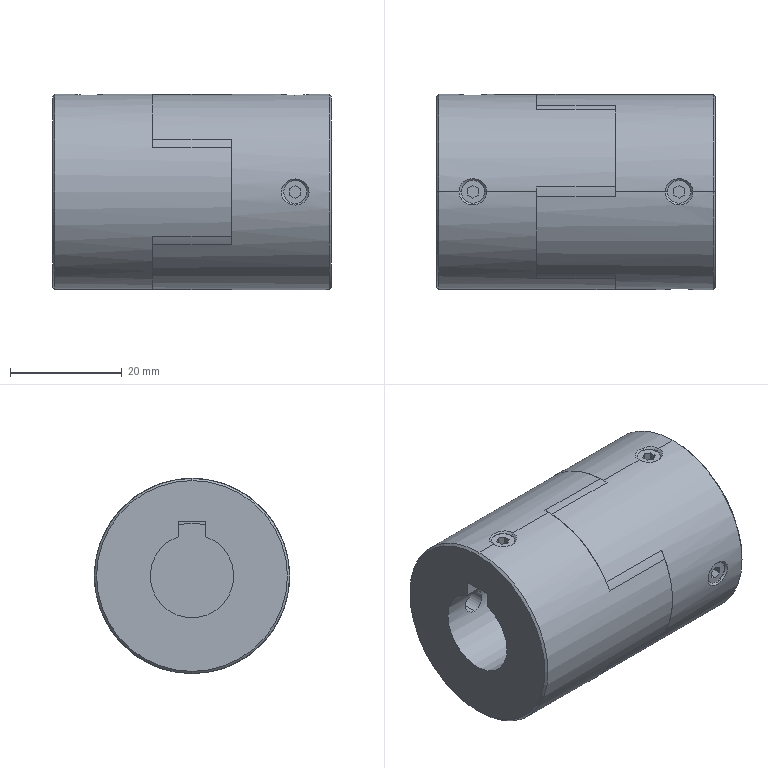Part | SolidWorks | features BaseBody 7 | 7 solids | 161 faces | box 50 x 35 x 35 mm | volume 38526 mm3 | cylinder 73 | plane 52 | cone 36 | commonest cylinder face diameters 19 x32 22 x12 35 x11 4.134 x8 5 x8 15 x2